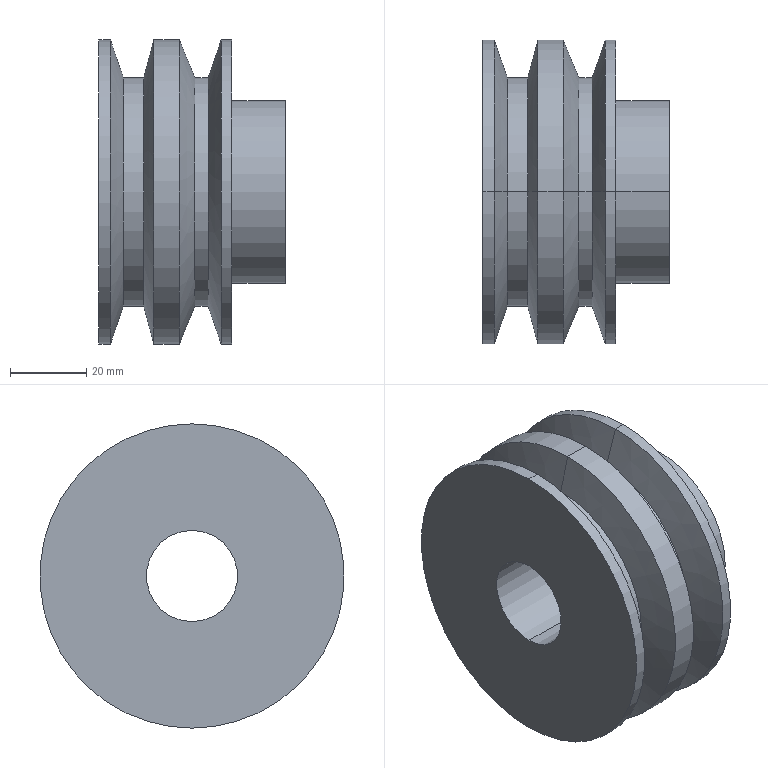Part | SolidWorks | features Revolution 1 | 1 solid | 25 faces | box 48.997 x 80 x 80 mm | volume 144144 mm3 | cylinder 14 | cone 8 | plane 3 | commonest cylinder face diameters 80 x6 60.183 x4 24 x2 48 x2
STEP:
#1=CARTESIAN_POINT('',(35.,0.,40.));
#2=VERTEX_POINT('',#1);
#3=CARTESIAN_POINT('',(35.,0.,-40.));
#4=VERTEX_POINT('',#3);
#5=CARTESIAN_POINT('',(35.,0.,0.));
#6=DIRECTION('',(-1.,0.,0.));
#7=DIRECTION('',(0.,0.,1.));
#8=AXIS2_PLACEMENT_3D('',#5,#6,#7);
#9=CIRCLE('',#8,40.);
#10=EDGE_CURVE('',#2,#4,#9,.T.);
#11=ORIENTED_EDGE('',*,*,#10,.T.);
#12=CARTESIAN_POINT('',(32.191,0.,-40.));
#13=VERTEX_POINT('',#12);
#14=CARTESIAN_POINT('',(0.,0.,-40.));
#15=DIRECTION('',(-1.,0.,0.));
#16=VECTOR('',#15,1000.);
#17=LINE('',#14,#16);
#18=EDGE_CURVE('',#4,#13,#17,.T.);
#19=ORIENTED_EDGE('',*,*,#18,.T.);
#20=CARTESIAN_POINT('',(32.191,0.,40.));
#21=VERTEX_POINT('',#20);
#22=CARTESIAN_POINT('',(32.191,0.,0.));
#23=DIRECTION('',(-1.,0.,0.));
#24=DIRECTION('',(0.,0.,1.));
#25=AXIS2_PLACEMENT_3D('',#22,#23,#24);
#26=CIRCLE('',#25,40.);
#27=EDGE_CURVE('',#21,#13,#26,.T.);
#28=ORIENTED_EDGE('',*,*,#27,.F.);
#29=CARTESIAN_POINT('',(0.,0.,40.));
#30=DIRECTION('',(-1.,0.,0.));
#31=VECTOR('',#30,1000.);
#32=LINE('',#29,#31);
#33=EDGE_CURVE('',#2,#21,#32,.T.);
#34=ORIENTED_EDGE('',*,*,#33,.F.);
#35=EDGE_LOOP('',(#11,#19,#28,#34));
#36=FACE_OUTER_BOUND('',#35,.T.);
#37=CARTESIAN_POINT('',(0.,0.,0.));
#38=DIRECTION('',(-1.,0.,0.));
#39=DIRECTION('',(0.,0.,1.));
#40=AXIS2_PLACEMENT_3D('',#37,#38,#39);
#41=CYLINDRICAL_SURFACE('',#40,40.);
#42=ADVANCED_FACE('',(#36),#41,.T.);
#43=CARTESIAN_POINT('',(28.775,0.,30.092));
#44=VERTEX_POINT('',#43);
#45=CARTESIAN_POINT('',(28.775,0.,-30.092));
#46=VERTEX_POINT('',#45);
#47=CARTESIAN_POINT('',(28.775,0.,0.));
#48=DIRECTION('',(-1.,0.,0.));
#49=DIRECTION('',(0.,0.,1.));
#50=AXIS2_PLACEMENT_3D('',#47,#48,#49);
#51=CIRCLE('',#50,30.092);
#52=EDGE_CURVE('',#44,#46,#51,.T.);
#53=ORIENTED_EDGE('',*,*,#52,.F.);
#54=CARTESIAN_POINT('',(32.191,0.,40.));
#55=DIRECTION('',(0.3259,0.,0.9454));
#56=VECTOR('',#55,1000.);
#57=LINE('',#54,#56);
#58=EDGE_CURVE('',#44,#21,#57,.T.);
#59=ORIENTED_EDGE('',*,*,#58,.T.);
#60=ORIENTED_EDGE('',*,*,#27,.T.);
#61=CARTESIAN_POINT('',(32.191,0.,-40.));
#62=DIRECTION('',(0.3259,0.,-0.9454));
#63=VECTOR('',#62,1000.);
#64=LINE('',#61,#63);
#65=EDGE_CURVE('',#46,#13,#64,.T.);
#66=ORIENTED_EDGE('',*,*,#65,.F.);
#67=EDGE_LOOP('',(#53,#59,#60,#66));
#68=FACE_OUTER_BOUND('',#67,.T.);
#69=CARTESIAN_POINT('',(32.191,0.,0.));
#70=DIRECTION('',(1.,0.,0.));
#71=DIRECTION('',(0.,0.,-1.));
#72=AXIS2_PLACEMENT_3D('',#69,#70,#71);
#73=CONICAL_SURFACE('',#72,40.,1.239);
#74=ADVANCED_FACE('',(#68),#73,.T.);
#75=ORIENTED_EDGE('',*,*,#52,.T.);
#76=CARTESIAN_POINT('',(25.228,0.,-30.092));
#77=VERTEX_POINT('',#76);
#78=CARTESIAN_POINT('',(0.,0.,-30.092));
#79=DIRECTION('',(-1.,0.,0.));
#80=VECTOR('',#79,1000.);
#81=LINE('',#78,#80);
#82=EDGE_CURVE('',#46,#77,#81,.T.);
#83=ORIENTED_EDGE('',*,*,#82,.T.);
#84=CARTESIAN_POINT('',(25.228,0.,30.092));
#85=VERTEX_POINT('',#84);
#86=CARTESIAN_POINT('',(25.228,0.,0.));
#87=DIRECTION('',(-1.,0.,0.));
#88=DIRECTION('',(0.,0.,1.));
#89=AXIS2_PLACEMENT_3D('',#86,#87,#88);
#90=CIRCLE('',#89,30.092);
#91=EDGE_CURVE('',#85,#77,#90,.T.);
#92=ORIENTED_EDGE('',*,*,#91,.F.);
#93=CARTESIAN_POINT('',(0.,0.,30.092));
#94=DIRECTION('',(-1.,0.,0.));
#95=VECTOR('',#94,1000.);
#96=LINE('',#93,#95);
#97=EDGE_CURVE('',#44,#85,#96,.T.);
#98=ORIENTED_EDGE('',*,*,#97,.F.);
#99=EDGE_LOOP('',(#75,#83,#92,#98));
#100=FACE_OUTER_BOUND('',#99,.T.);
#101=CARTESIAN_POINT('',(0.,0.,0.));
#102=DIRECTION('',(-1.,0.,0.));
#103=DIRECTION('',(0.,0.,1.));
#104=AXIS2_PLACEMENT_3D('',#101,#102,#103);
#105=CYLINDRICAL_SURFACE('',#104,30.092);
#106=ADVANCED_FACE('',(#100),#105,.T.);
#107=ORIENTED_EDGE('',*,*,#91,.T.);
#108=CARTESIAN_POINT('',(21.155,0.,-40.));
#109=VERTEX_POINT('',#108);
#110=CARTESIAN_POINT('',(25.228,0.,-30.092));
#111=DIRECTION('',(-0.3802,0.,-0.9249));
#112=VECTOR('',#111,1000.);
#113=LINE('',#110,#112);
#114=EDGE_CURVE('',#77,#109,#113,.T.);
#115=ORIENTED_EDGE('',*,*,#114,.T.);
#116=CARTESIAN_POINT('',(21.155,0.,40.));
#117=VERTEX_POINT('',#116);
#118=CARTESIAN_POINT('',(21.155,0.,0.));
#119=DIRECTION('',(-1.,0.,0.));
#120=DIRECTION('',(0.,0.,1.));
#121=AXIS2_PLACEMENT_3D('',#118,#119,#120);
#122=CIRCLE('',#121,40.);
#123=EDGE_CURVE('',#117,#109,#122,.T.);
#124=ORIENTED_EDGE('',*,*,#123,.F.);
#125=CARTESIAN_POINT('',(25.228,0.,30.092));
#126=DIRECTION('',(-0.3802,0.,0.9249));
#127=VECTOR('',#126,1000.);
#128=LINE('',#125,#127);
#129=EDGE_CURVE('',#85,#117,#128,.T.);
#130=ORIENTED_EDGE('',*,*,#129,.F.);
#131=EDGE_LOOP('',(#107,#115,#124,#130));
#132=FACE_OUTER_BOUND('',#131,.T.);
#133=CARTESIAN_POINT('',(25.228,0.,0.));
#134=DIRECTION('',(-1.,0.,0.));
#135=DIRECTION('',(0.,0.,1.));
#136=AXIS2_PLACEMENT_3D('',#133,#134,#135);
#137=CONICAL_SURFACE('',#136,30.092,1.181);
#138=ADVANCED_FACE('',(#132),#137,.T.);
#139=ORIENTED_EDGE('',*,*,#123,.T.);
#140=CARTESIAN_POINT('',(14.455,0.,-40.));
#141=VERTEX_POINT('',#140);
#142=CARTESIAN_POINT('',(0.,0.,-40.));
#143=DIRECTION('',(-1.,0.,0.));
#144=VECTOR('',#143,1000.);
#145=LINE('',#142,#144);
#146=EDGE_CURVE('',#109,#141,#145,.T.);
#147=ORIENTED_EDGE('',*,*,#146,.T.);
#148=CARTESIAN_POINT('',(14.455,0.,40.));
#149=VERTEX_POINT('',#148);
#150=CARTESIAN_POINT('',(14.455,0.,0.));
#151=DIRECTION('',(-1.,0.,0.));
#152=DIRECTION('',(0.,0.,1.));
#153=AXIS2_PLACEMENT_3D('',#150,#151,#152);
#154=CIRCLE('',#153,40.);
#155=EDGE_CURVE('',#149,#141,#154,.T.);
#156=ORIENTED_EDGE('',*,*,#155,.F.);
#157=CARTESIAN_POINT('',(0.,0.,40.));
#158=DIRECTION('',(-1.,0.,0.));
#159=VECTOR('',#158,1000.);
#160=LINE('',#157,#159);
#161=EDGE_CURVE('',#117,#149,#160,.T.);
#162=ORIENTED_EDGE('',*,*,#161,.F.);
#163=EDGE_LOOP('',(#139,#147,#156,#162));
#164=FACE_OUTER_BOUND('',#163,.T.);
#165=CARTESIAN_POINT('',(0.,0.,0.));
#166=DIRECTION('',(-1.,0.,0.));
#167=DIRECTION('',(0.,0.,1.));
#168=AXIS2_PLACEMENT_3D('',#165,#166,#167);
#169=CYLINDRICAL_SURFACE('',#168,40.);
#170=ADVANCED_FACE('',(#164),#169,.T.);
#171=CARTESIAN_POINT('',(11.828,0.,30.092));
#172=VERTEX_POINT('',#171);
#173=CARTESIAN_POINT('',(11.828,0.,-30.092));
#174=VERTEX_POINT('',#173);
#175=CARTESIAN_POINT('',(11.828,0.,0.));
#176=DIRECTION('',(-1.,0.,0.));
#177=DIRECTION('',(0.,0.,1.));
#178=AXIS2_PLACEMENT_3D('',#175,#176,#177);
#179=CIRCLE('',#178,30.092);
#180=EDGE_CURVE('',#172,#174,#179,.T.);
#181=ORIENTED_EDGE('',*,*,#180,.F.);
#182=CARTESIAN_POINT('',(14.455,0.,40.));
#183=DIRECTION('',(0.2563,0.,0.9666));
#184=VECTOR('',#183,1000.);
#185=LINE('',#182,#184);
#186=EDGE_CURVE('',#172,#149,#185,.T.);
#187=ORIENTED_EDGE('',*,*,#186,.T.);
#188=ORIENTED_EDGE('',*,*,#155,.T.);
#189=CARTESIAN_POINT('',(14.455,0.,-40.));
#190=DIRECTION('',(0.2563,0.,-0.9666));
#191=VECTOR('',#190,1000.);
#192=LINE('',#189,#191);
#193=EDGE_CURVE('',#174,#141,#192,.T.);
#194=ORIENTED_EDGE('',*,*,#193,.F.);
#195=EDGE_LOOP('',(#181,#187,#188,#194));
#196=FACE_OUTER_BOUND('',#195,.T.);
#197=CARTESIAN_POINT('',(14.455,0.,0.));
#198=DIRECTION('',(1.,0.,0.));
#199=DIRECTION('',(0.,0.,-1.));
#200=AXIS2_PLACEMENT_3D('',#197,#198,#199);
#201=CONICAL_SURFACE('',#200,40.,1.312);
#202=ADVANCED_FACE('',(#196),#201,.T.);
#203=ORIENTED_EDGE('',*,*,#180,.T.);
#204=CARTESIAN_POINT('',(6.442,0.,-30.092));
#205=VERTEX_POINT('',#204);
#206=CARTESIAN_POINT('',(0.,0.,-30.092));
#207=DIRECTION('',(-1.,0.,0.));
#208=VECTOR('',#207,1000.);
#209=LINE('',#206,#208);
#210=EDGE_CURVE('',#174,#205,#209,.T.);
#211=ORIENTED_EDGE('',*,*,#210,.T.);
#212=CARTESIAN_POINT('',(6.442,0.,30.092));
#213=VERTEX_POINT('',#212);
#214=CARTESIAN_POINT('',(6.442,0.,0.));
#215=DIRECTION('',(-1.,0.,0.));
#216=DIRECTION('',(0.,0.,1.));
#217=AXIS2_PLACEMENT_3D('',#214,#215,#216);
#218=CIRCLE('',#217,30.092);
#219=EDGE_CURVE('',#213,#205,#218,.T.);
#220=ORIENTED_EDGE('',*,*,#219,.F.);
#221=CARTESIAN_POINT('',(0.,0.,30.092));
#222=DIRECTION('',(-1.,0.,0.));
#223=VECTOR('',#222,1000.);
#224=LINE('',#221,#223);
#225=EDGE_CURVE('',#172,#213,#224,.T.);
#226=ORIENTED_EDGE('',*,*,#225,.F.);
#227=EDGE_LOOP('',(#203,#211,#220,#226));
#228=FACE_OUTER_BOUND('',#227,.T.);
#229=CARTESIAN_POINT('',(0.,0.,0.));
#230=DIRECTION('',(-1.,0.,0.));
#231=DIRECTION('',(0.,0.,1.));
#232=AXIS2_PLACEMENT_3D('',#229,#230,#231);
#233=CYLINDRICAL_SURFACE('',#232,30.092);
#234=ADVANCED_FACE('',(#228),#233,.T.);
#235=ORIENTED_EDGE('',*,*,#219,.T.);
#236=CARTESIAN_POINT('',(3.026,0.,-40.));
#237=VERTEX_POINT('',#236);
#238=CARTESIAN_POINT('',(6.442,0.,-30.092));
#239=DIRECTION('',(-0.3259,0.,-0.9454));
#240=VECTOR('',#239,1000.);
#241=LINE('',#238,#240);
#242=EDGE_CURVE('',#205,#237,#241,.T.);
#243=ORIENTED_EDGE('',*,*,#242,.T.);
#244=CARTESIAN_POINT('',(3.026,0.,40.));
#245=VERTEX_POINT('',#244);
#246=CARTESIAN_POINT('',(3.026,0.,0.));
#247=DIRECTION('',(-1.,0.,0.));
#248=DIRECTION('',(0.,0.,1.));
#249=AXIS2_PLACEMENT_3D('',#246,#247,#248);
#250=CIRCLE('',#249,40.);
#251=EDGE_CURVE('',#245,#237,#250,.T.);
#252=ORIENTED_EDGE('',*,*,#251,.F.);
#253=CARTESIAN_POINT('',(6.442,0.,30.092));
#254=DIRECTION('',(-0.3259,0.,0.9454));
#255=VECTOR('',#254,1000.);
#256=LINE('',#253,#255);
#257=EDGE_CURVE('',#213,#245,#256,.T.);
#258=ORIENTED_EDGE('',*,*,#257,.F.);
#259=EDGE_LOOP('',(#235,#243,#252,#258));
#260=FACE_OUTER_BOUND('',#259,.T.);
#261=CARTESIAN_POINT('',(6.442,0.,0.));
#262=DIRECTION('',(-1.,0.,0.));
#263=DIRECTION('',(0.,0.,1.));
#264=AXIS2_PLACEMENT_3D('',#261,#262,#263);
#265=CONICAL_SURFACE('',#264,30.092,1.239);
#266=ADVANCED_FACE('',(#260),#265,.T.);
#267=ORIENTED_EDGE('',*,*,#251,.T.);
#268=CARTESIAN_POINT('',(0.,0.,-40.));
#269=VERTEX_POINT('',#268);
#270=CARTESIAN_POINT('',(0.,0.,-40.));
#271=DIRECTION('',(-1.,0.,0.));
#272=VECTOR('',#271,1000.);
#273=LINE('',#270,#272);
#274=EDGE_CURVE('',#237,#269,#273,.T.);
#275=ORIENTED_EDGE('',*,*,#274,.T.);
#276=CARTESIAN_POINT('',(0.,0.,40.));
#277=VERTEX_POINT('',#276);
#278=CARTESIAN_POINT('',(0.,0.,0.));
#279=DIRECTION('',(-1.,0.,0.));
#280=DIRECTION('',(0.,0.,1.));
#281=AXIS2_PLACEMENT_3D('',#278,#279,#280);
#282=CIRCLE('',#281,40.);
#283=EDGE_CURVE('',#277,#269,#282,.T.);
#284=ORIENTED_EDGE('',*,*,#283,.F.);
#285=CARTESIAN_POINT('',(0.,0.,40.));
#286=DIRECTION('',(-1.,0.,0.));
#287=VECTOR('',#286,1000.);
#288=LINE('',#285,#287);
#289=EDGE_CURVE('',#245,#277,#288,.T.);
#290=ORIENTED_EDGE('',*,*,#289,.F.);
#291=EDGE_LOOP('',(#267,#275,#284,#290));
#292=FACE_OUTER_BOUND('',#291,.T.);
#293=CARTESIAN_POINT('',(0.,0.,0.));
#294=DIRECTION('',(-1.,0.,0.));
#295=DIRECTION('',(0.,0.,1.));
#296=AXIS2_PLACEMENT_3D('',#293,#294,#295);
#297=CYLINDRICAL_SURFACE('',#296,40.);
#298=ADVANCED_FACE('',(#292),#297,.T.);
#299=CARTESIAN_POINT('',(48.997,0.,-12.));
#300=VERTEX_POINT('',#299);
#301=CARTESIAN_POINT('',(48.997,0.,12.));
#302=VERTEX_POINT('',#301);
#303=CARTESIAN_POINT('',(48.997,0.,0.));
#304=DIRECTION('',(-1.,0.,0.));
#305=DIRECTION('',(0.,0.,1.));
#306=AXIS2_PLACEMENT_3D('',#303,#304,#305);
#307=CIRCLE('',#306,12.);
#308=EDGE_CURVE('',#300,#302,#307,.T.);
#309=ORIENTED_EDGE('',*,*,#308,.F.);
#310=CARTESIAN_POINT('',(0.,0.,-12.));
#311=VERTEX_POINT('',#310);
#312=CARTESIAN_POINT('',(0.,0.,-12.));
#313=DIRECTION('',(-1.,0.,0.));
#314=VECTOR('',#313,1000.);
#315=LINE('',#312,#314);
#316=EDGE_CURVE('',#300,#311,#315,.T.);
#317=ORIENTED_EDGE('',*,*,#316,.T.);
#318=CARTESIAN_POINT('',(0.,0.,12.));
#319=VERTEX_POINT('',#318);
#320=CARTESIAN_POINT('',(0.,0.,0.));
#321=DIRECTION('',(-1.,0.,0.));
#322=DIRECTION('',(0.,0.,1.));
#323=AXIS2_PLACEMENT_3D('',#320,#321,#322);
#324=CIRCLE('',#323,12.);
#325=EDGE_CURVE('',#311,#319,#324,.T.);
#326=ORIENTED_EDGE('',*,*,#325,.T.);
#327=CARTESIAN_POINT('',(0.,0.,12.));
#328=DIRECTION('',(-1.,0.,0.));
#329=VECTOR('',#328,1000.);
#330=LINE('',#327,#329);
#331=EDGE_CURVE('',#302,#319,#330,.T.);
#332=ORIENTED_EDGE('',*,*,#331,.F.);
#333=EDGE_LOOP('',(#309,#317,#326,#332));
#334=FACE_OUTER_BOUND('',#333,.T.);
#335=CARTESIAN_POINT('',(0.,0.,0.));
#336=DIRECTION('',(-1.,0.,0.));
#337=DIRECTION('',(0.,0.,1.));
#338=AXIS2_PLACEMENT_3D('',#335,#336,#337);
#339=CYLINDRICAL_SURFACE('',#338,12.);
#340=ADVANCED_FACE('',(#334),#339,.F.);
#341=CARTESIAN_POINT('',(48.997,0.,24.));
#342=VERTEX_POINT('',#341);
#343=CARTESIAN_POINT('',(48.997,0.,-24.));
#344=VERTEX_POINT('',#343);
#345=CARTESIAN_POINT('',(48.997,0.,0.));
#346=DIRECTION('',(-1.,0.,0.));
#347=DIRECTION('',(0.,0.,1.));
#348=AXIS2_PLACEMENT_3D('',#345,#346,#347);
#349=CIRCLE('',#348,24.);
#350=EDGE_CURVE('',#342,#344,#349,.T.);
#351=ORIENTED_EDGE('',*,*,#350,.T.);
#352=CARTESIAN_POINT('',(35.,0.,-24.));
#353=VERTEX_POINT('',#352);
#354=CARTESIAN_POINT('',(0.,0.,-24.));
#355=DIRECTION('',(-1.,0.,0.));
#356=VECTOR('',#355,1000.);
#357=LINE('',#354,#356);
#358=EDGE_CURVE('',#344,#353,#357,.T.);
#359=ORIENTED_EDGE('',*,*,#358,.T.);
#360=CARTESIAN_POINT('',(35.,0.,24.));
#361=VERTEX_POINT('',#360);
#362=CARTESIAN_POINT('',(35.,0.,0.));
#363=DIRECTION('',(-1.,0.,0.));
#364=DIRECTION('',(0.,0.,1.));
#365=AXIS2_PLACEMENT_3D('',#362,#363,#364);
#366=CIRCLE('',#365,24.);
#367=EDGE_CURVE('',#361,#353,#366,.T.);
#368=ORIENTED_EDGE('',*,*,#367,.F.);
#369=CARTESIAN_POINT('',(0.,0.,24.));
#370=DIRECTION('',(-1.,0.,0.));
#371=VECTOR('',#370,1000.);
#372=LINE('',#369,#371);
#373=EDGE_CURVE('',#342,#361,#372,.T.);
#374=ORIENTED_EDGE('',*,*,#373,.F.);
#375=EDGE_LOOP('',(#351,#359,#368,#374));
#376=FACE_OUTER_BOUND('',#375,.T.);
#377=CARTESIAN_POINT('',(0.,0.,0.));
#378=DIRECTION('',(-1.,0.,0.));
#379=DIRECTION('',(0.,0.,1.));
#380=AXIS2_PLACEMENT_3D('',#377,#378,#379);
#381=CYLINDRICAL_SURFACE('',#380,24.);
#382=ADVANCED_FACE('',(#376),#381,.T.);
#383=ORIENTED_EDGE('',*,*,#358,.F.);
#384=CARTESIAN_POINT('',(48.997,0.,0.));
#385=DIRECTION('',(-1.,0.,0.));
#386=DIRECTION('',(0.,0.,1.));
#387=AXIS2_PLACEMENT_3D('',#384,#385,#386);
#388=CIRCLE('',#387,24.);
#389=EDGE_CURVE('',#344,#342,#388,.T.);
#390=ORIENTED_EDGE('',*,*,#389,.T.);
#391=ORIENTED_EDGE('',*,*,#373,.T.);
#392=CARTESIAN_POINT('',(35.,0.,0.));
#393=DIRECTION('',(-1.,0.,0.));
#394=DIRECTION('',(0.,0.,1.));
#395=AXIS2_PLACEMENT_3D('',#392,#393,#394);
#396=CIRCLE('',#395,24.);
#397=EDGE_CURVE('',#353,#361,#396,.T.);
#398=ORIENTED_EDGE('',*,*,#397,.F.);
#399=EDGE_LOOP('',(#383,#390,#391,#398));
#400=FACE_OUTER_BOUND('',#399,.T.);
#401=CARTESIAN_POINT('',(0.,0.,0.));
#402=DIRECTION('',(-1.,0.,0.));
#403=DIRECTION('',(0.,0.,1.));
#404=AXIS2_PLACEMENT_3D('',#401,#402,#403);
#405=CYLINDRICAL_SURFACE('',#404,24.);
#406=ADVANCED_FACE('',(#400),#405,.T.);
#407=ORIENTED_EDGE('',*,*,#350,.F.);
#408=ORIENTED_EDGE('',*,*,#389,.F.);
#409=EDGE_LOOP('',(#407,#408));
#410=FACE_OUTER_BOUND('',#409,.T.);
#411=CARTESIAN_POINT('',(48.997,0.,0.));
#412=DIRECTION('',(-1.,0.,0.));
#413=DIRECTION('',(0.,0.,1.));
#414=AXIS2_PLACEMENT_3D('',#411,#412,#413);
#415=CIRCLE('',#414,12.);
#416=EDGE_CURVE('',#302,#300,#415,.T.);
#417=ORIENTED_EDGE('',*,*,#416,.T.);
#418=ORIENTED_EDGE('',*,*,#308,.T.);
#419=EDGE_LOOP('',(#417,#418));
#420=FACE_BOUND('',#419,.T.);
#421=CARTESIAN_POINT('',(48.997,0.,-24.));
#422=DIRECTION('',(-1.,0.,0.));
#423=DIRECTION('',(0.,0.,1.));
#424=AXIS2_PLACEMENT_3D('',#421,#422,#423);
#425=PLANE('',#424);
#426=ADVANCED_FACE('',(#410,#420),#425,.F.);
#427=ORIENTED_EDGE('',*,*,#316,.F.);
#428=ORIENTED_EDGE('',*,*,#416,.F.);
#429=ORIENTED_EDGE('',*,*,#331,.T.);
#430=CARTESIAN_POINT('',(0.,0.,0.));
#431=DIRECTION('',(-1.,0.,0.));
#432=DIRECTION('',(0.,0.,1.));
#433=AXIS2_PLACEMENT_3D('',#430,#431,#432);
#434=CIRCLE('',#433,12.);
#435=EDGE_CURVE('',#319,#311,#434,.T.);
#436=ORIENTED_EDGE('',*,*,#435,.T.);
#437=EDGE_LOOP('',(#427,#428,#429,#436));
#438=FACE_OUTER_BOUND('',#437,.T.);
#439=CARTESIAN_POINT('',(0.,0.,0.));
#440=DIRECTION('',(-1.,0.,0.));
#441=DIRECTION('',(0.,0.,1.));
#442=AXIS2_PLACEMENT_3D('',#439,#440,#441);
#443=CYLINDRICAL_SURFACE('',#442,12.);
#444=ADVANCED_FACE('',(#438),#443,.F.);
#445=ORIENTED_EDGE('',*,*,#435,.F.);
#446=ORIENTED_EDGE('',*,*,#325,.F.);
#447=EDGE_LOOP('',(#445,#446));
#448=FACE_BOUND('',#447,.T.);
#449=ORIENTED_EDGE('',*,*,#283,.T.);
#450=CARTESIAN_POINT('',(0.,0.,0.));
#451=DIRECTION('',(-1.,0.,0.));
#452=DIRECTION('',(0.,0.,1.));
#453=AXIS2_PLACEMENT_3D('',#450,#451,#452);
#454=CIRCLE('',#453,40.);
#455=EDGE_CURVE('',#269,#277,#454,.T.);
#456=ORIENTED_EDGE('',*,*,#455,.T.);
#457=EDGE_LOOP('',(#449,#456));
#458=FACE_OUTER_BOUND('',#457,.T.);
#459=CARTESIAN_POINT('',(0.,0.,-12.));
#460=DIRECTION('',(1.,0.,0.));
#461=DIRECTION('',(0.,0.,-1.));
#462=AXIS2_PLACEMENT_3D('',#459,#460,#461);
#463=PLANE('',#462);
#464=ADVANCED_FACE('',(#448,#458),#463,.F.);
#465=ORIENTED_EDGE('',*,*,#274,.F.);
#466=CARTESIAN_POINT('',(3.026,0.,0.));
#467=DIRECTION('',(-1.,0.,0.));
#468=DIRECTION('',(0.,0.,1.));
#469=AXIS2_PLACEMENT_3D('',#466,#467,#468);
#470=CIRCLE('',#469,40.);
#471=EDGE_CURVE('',#237,#245,#470,.T.);
#472=ORIENTED_EDGE('',*,*,#471,.T.);
#473=ORIENTED_EDGE('',*,*,#289,.T.);
#474=ORIENTED_EDGE('',*,*,#455,.F.);
#475=EDGE_LOOP('',(#465,#472,#473,#474));
#476=FACE_OUTER_BOUND('',#475,.T.);
#477=CARTESIAN_POINT('',(0.,0.,0.));
#478=DIRECTION('',(-1.,0.,0.));
#479=DIRECTION('',(0.,0.,1.));
#480=AXIS2_PLACEMENT_3D('',#477,#478,#479);
#481=CYLINDRICAL_SURFACE('',#480,40.);
#482=ADVANCED_FACE('',(#476),#481,.T.);
#483=ORIENTED_EDGE('',*,*,#242,.F.);
#484=CARTESIAN_POINT('',(6.442,0.,0.));
#485=DIRECTION('',(-1.,0.,0.));
#486=DIRECTION('',(0.,0.,1.));
#487=AXIS2_PLACEMENT_3D('',#484,#485,#486);
#488=CIRCLE('',#487,30.092);
#489=EDGE_CURVE('',#205,#213,#488,.T.);
#490=ORIENTED_EDGE('',*,*,#489,.T.);
#491=ORIENTED_EDGE('',*,*,#257,.T.);
#492=ORIENTED_EDGE('',*,*,#471,.F.);
#493=EDGE_LOOP('',(#483,#490,#491,#492));
#494=FACE_OUTER_BOUND('',#493,.T.);
#495=CARTESIAN_POINT('',(6.442,0.,0.));
#496=DIRECTION('',(-1.,0.,0.));
#497=DIRECTION('',(0.,0.,1.));
#498=AXIS2_PLACEMENT_3D('',#495,#496,#497);
#499=CONICAL_SURFACE('',#498,30.092,1.239);
#500=ADVANCED_FACE('',(#494),#499,.T.);
#501=ORIENTED_EDGE('',*,*,#210,.F.);
#502=CARTESIAN_POINT('',(11.828,0.,0.));
#503=DIRECTION('',(-1.,0.,0.));
#504=DIRECTION('',(0.,0.,1.));
#505=AXIS2_PLACEMENT_3D('',#502,#503,#504);
#506=CIRCLE('',#505,30.092);
#507=EDGE_CURVE('',#174,#172,#506,.T.);
#508=ORIENTED_EDGE('',*,*,#507,.T.);
#509=ORIENTED_EDGE('',*,*,#225,.T.);
#510=ORIENTED_EDGE('',*,*,#489,.F.);
#511=EDGE_LOOP('',(#501,#508,#509,#510));
#512=FACE_OUTER_BOUND('',#511,.T.);
#513=CARTESIAN_POINT('',(0.,0.,0.));
#514=DIRECTION('',(-1.,0.,0.));
#515=DIRECTION('',(0.,0.,1.));
#516=AXIS2_PLACEMENT_3D('',#513,#514,#515);
#517=CYLINDRICAL_SURFACE('',#516,30.092);
#518=ADVANCED_FACE('',(#512),#517,.T.);
#519=ORIENTED_EDGE('',*,*,#186,.F.);
#520=ORIENTED_EDGE('',*,*,#507,.F.);
#521=ORIENTED_EDGE('',*,*,#193,.T.);
#522=CARTESIAN_POINT('',(14.455,0.,0.));
#523=DIRECTION('',(-1.,0.,0.));
#524=DIRECTION('',(0.,0.,1.));
#525=AXIS2_PLACEMENT_3D('',#522,#523,#524);
#526=CIRCLE('',#525,40.);
#527=EDGE_CURVE('',#141,#149,#526,.T.);
#528=ORIENTED_EDGE('',*,*,#527,.T.);
#529=EDGE_LOOP('',(#519,#520,#521,#528));
#530=FACE_OUTER_BOUND('',#529,.T.);
#531=CARTESIAN_POINT('',(14.455,0.,0.));
#532=DIRECTION('',(1.,0.,0.));
#533=DIRECTION('',(0.,0.,-1.));
#534=AXIS2_PLACEMENT_3D('',#531,#532,#533);
#535=CONICAL_SURFACE('',#534,40.,1.312);
#536=ADVANCED_FACE('',(#530),#535,.T.);
#537=ORIENTED_EDGE('',*,*,#146,.F.);
#538=CARTESIAN_POINT('',(21.155,0.,0.));
#539=DIRECTION('',(-1.,0.,0.));
#540=DIRECTION('',(0.,0.,1.));
#541=AXIS2_PLACEMENT_3D('',#538,#539,#540);
#542=CIRCLE('',#541,40.);
#543=EDGE_CURVE('',#109,#117,#542,.T.);
#544=ORIENTED_EDGE('',*,*,#543,.T.);
#545=ORIENTED_EDGE('',*,*,#161,.T.);
#546=ORIENTED_EDGE('',*,*,#527,.F.);
#547=EDGE_LOOP('',(#537,#544,#545,#546));
#548=FACE_OUTER_BOUND('',#547,.T.);
#549=CARTESIAN_POINT('',(0.,0.,0.));
#550=DIRECTION('',(-1.,0.,0.));
#551=DIRECTION('',(0.,0.,1.));
#552=AXIS2_PLACEMENT_3D('',#549,#550,#551);
#553=CYLINDRICAL_SURFACE('',#552,40.);
#554=ADVANCED_FACE('',(#548),#553,.T.);
#555=ORIENTED_EDGE('',*,*,#114,.F.);
#556=CARTESIAN_POINT('',(25.228,0.,0.));
#557=DIRECTION('',(-1.,0.,0.));
#558=DIRECTION('',(0.,0.,1.));
#559=AXIS2_PLACEMENT_3D('',#556,#557,#558);
#560=CIRCLE('',#559,30.092);
#561=EDGE_CURVE('',#77,#85,#560,.T.);
#562=ORIENTED_EDGE('',*,*,#561,.T.);
#563=ORIENTED_EDGE('',*,*,#129,.T.);
#564=ORIENTED_EDGE('',*,*,#543,.F.);
#565=EDGE_LOOP('',(#555,#562,#563,#564));
#566=FACE_OUTER_BOUND('',#565,.T.);
#567=CARTESIAN_POINT('',(25.228,0.,0.));
#568=DIRECTION('',(-1.,0.,0.));
#569=DIRECTION('',(0.,0.,1.));
#570=AXIS2_PLACEMENT_3D('',#567,#568,#569);
#571=CONICAL_SURFACE('',#570,30.092,1.181);
#572=ADVANCED_FACE('',(#566),#571,.T.);
#573=ORIENTED_EDGE('',*,*,#82,.F.);
#574=CARTESIAN_POINT('',(28.775,0.,0.));
#575=DIRECTION('',(-1.,0.,0.));
#576=DIRECTION('',(0.,0.,1.));
#577=AXIS2_PLACEMENT_3D('',#574,#575,#576);
#578=CIRCLE('',#577,30.092);
#579=EDGE_CURVE('',#46,#44,#578,.T.);
#580=ORIENTED_EDGE('',*,*,#579,.T.);
#581=ORIENTED_EDGE('',*,*,#97,.T.);
#582=ORIENTED_EDGE('',*,*,#561,.F.);
#583=EDGE_LOOP('',(#573,#580,#581,#582));
#584=FACE_OUTER_BOUND('',#583,.T.);
#585=CARTESIAN_POINT('',(0.,0.,0.));
#586=DIRECTION('',(-1.,0.,0.));
#587=DIRECTION('',(0.,0.,1.));
#588=AXIS2_PLACEMENT_3D('',#585,#586,#587);
#589=CYLINDRICAL_SURFACE('',#588,30.092);
#590=ADVANCED_FACE('',(#584),#589,.T.);
#591=ORIENTED_EDGE('',*,*,#58,.F.);
#592=ORIENTED_EDGE('',*,*,#579,.F.);
#593=ORIENTED_EDGE('',*,*,#65,.T.);
#594=CARTESIAN_POINT('',(32.191,0.,0.));
#595=DIRECTION('',(-1.,0.,0.));
#596=DIRECTION('',(0.,0.,1.));
#597=AXIS2_PLACEMENT_3D('',#594,#595,#596);
#598=CIRCLE('',#597,40.);
#599=EDGE_CURVE('',#13,#21,#598,.T.);
#600=ORIENTED_EDGE('',*,*,#599,.T.);
#601=EDGE_LOOP('',(#591,#592,#593,#600));
#602=FACE_OUTER_BOUND('',#601,.T.);
#603=CARTESIAN_POINT('',(32.191,0.,0.));
#604=DIRECTION('',(1.,0.,0.));
#605=DIRECTION('',(0.,0.,-1.));
#606=AXIS2_PLACEMENT_3D('',#603,#604,#605);
#607=CONICAL_SURFACE('',#606,40.,1.239);
#608=ADVANCED_FACE('',(#602),#607,.T.);
#609=ORIENTED_EDGE('',*,*,#18,.F.);
#610=CARTESIAN_POINT('',(35.,0.,0.));
#611=DIRECTION('',(-1.,0.,0.));
#612=DIRECTION('',(0.,0.,1.));
#613=AXIS2_PLACEMENT_3D('',#610,#611,#612);
#614=CIRCLE('',#613,40.);
#615=EDGE_CURVE('',#4,#2,#614,.T.);
#616=ORIENTED_EDGE('',*,*,#615,.T.);
#617=ORIENTED_EDGE('',*,*,#33,.T.);
#618=ORIENTED_EDGE('',*,*,#599,.F.);
#619=EDGE_LOOP('',(#609,#616,#617,#618));
#620=FACE_OUTER_BOUND('',#619,.T.);
#621=CARTESIAN_POINT('',(0.,0.,0.));
#622=DIRECTION('',(-1.,0.,0.));
#623=DIRECTION('',(0.,0.,1.));
#624=AXIS2_PLACEMENT_3D('',#621,#622,#623);
#625=CYLINDRICAL_SURFACE('',#624,40.);
#626=ADVANCED_FACE('',(#620),#625,.T.);
#627=ORIENTED_EDGE('',*,*,#10,.F.);
#628=ORIENTED_EDGE('',*,*,#615,.F.);
#629=EDGE_LOOP('',(#627,#628));
#630=FACE_OUTER_BOUND('',#629,.T.);
#631=ORIENTED_EDGE('',*,*,#367,.T.);
#632=ORIENTED_EDGE('',*,*,#397,.T.);
#633=EDGE_LOOP('',(#631,#632));
#634=FACE_BOUND('',#633,.T.);
#635=CARTESIAN_POINT('',(35.,0.,-40.));
#636=DIRECTION('',(-1.,0.,0.));
#637=DIRECTION('',(0.,0.,1.));
#638=AXIS2_PLACEMENT_3D('',#635,#636,#637);
#639=PLANE('',#638);
#640=ADVANCED_FACE('',(#630,#634),#639,.F.);
#641=CLOSED_SHELL('',(#42,#74,#106,#138,#170,#202,#234,#266,#298,#340,#382,#406,#426,#444,#464,#482,#500,#518,#536,#554,#572,#590,#608,#626,#640));
#642=MANIFOLD_SOLID_BREP('',#641);
#643=CARTESIAN_POINT('',(0.,0.,0.));
#644=DIRECTION('',(0.,0.,1.));
#645=DIRECTION('',(1.,0.,0.));
#646=AXIS2_PLACEMENT_3D('',#643,#644,#645);
#647=(LENGTH_UNIT()NAMED_UNIT(*)SI_UNIT(.MILLI.,.METRE.));
#648=UNCERTAINTY_MEASURE_WITH_UNIT(LENGTH_MEASURE(0.00001),#647,'','');
#649=(NAMED_UNIT(*)PLANE_ANGLE_UNIT()SI_UNIT($,.RADIAN.));
#650=(NAMED_UNIT(*)SI_UNIT($,.STERADIAN.)SOLID_ANGLE_UNIT());
#651=(GEOMETRIC_REPRESENTATION_CONTEXT(3)GLOBAL_UNCERTAINTY_ASSIGNED_CONTEXT((#648))GLOBAL_UNIT_ASSIGNED_CONTEXT((#647,#649,#650))REPRESENTATION_CONTEXT('',''));
#652=ADVANCED_BREP_SHAPE_REPRESENTATION('',(#642,#646),#651);